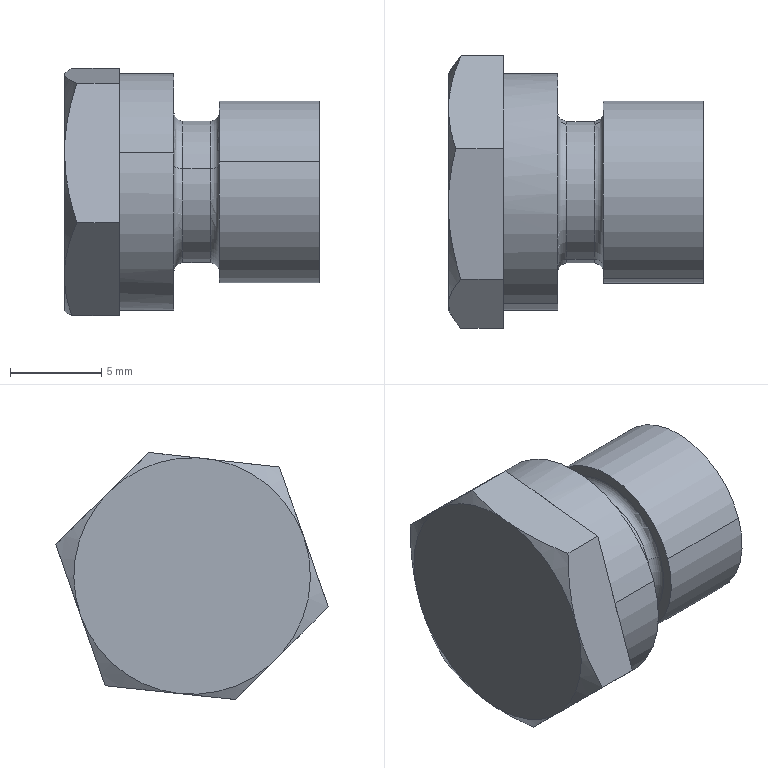Part | SolidWorks | features BaseBody 1 | 1 solid | 34 faces | box 14 x 14.972 x 13.575 mm | volume 1390 mm3 | plane 18 | cylinder 6 | cone 6 | torus 4 | commonest cylinder face diameters 7.8 x2 10 x2 13 x2
STEP:
#1=CARTESIAN_POINT('',(-79.963,84.032,-204.194));
#2=VERTEX_POINT('',#1);
#3=CARTESIAN_POINT('',(-79.963,71.76,-199.906));
#4=VERTEX_POINT('',#3);
#5=CARTESIAN_POINT('',(-79.963,77.896,-202.05));
#6=DIRECTION('',(1.,0.,0.));
#7=DIRECTION('',(0.,0.944,-0.3299));
#8=AXIS2_PLACEMENT_3D('',#5,#6,#7);
#9=CIRCLE('',#8,6.5);
#10=EDGE_CURVE('',#2,#4,#9,.T.);
#11=ORIENTED_EDGE('',*,*,#10,.F.);
#12=CARTESIAN_POINT('',(-82.963,84.032,-204.194));
#13=VERTEX_POINT('',#12);
#14=CARTESIAN_POINT('',(-79.963,84.032,-204.194));
#15=DIRECTION('',(-1.,0.,0.));
#16=VECTOR('',#15,1000.);
#17=LINE('',#14,#16);
#18=EDGE_CURVE('',#2,#13,#17,.T.);
#19=ORIENTED_EDGE('',*,*,#18,.T.);
#20=CARTESIAN_POINT('',(-82.963,82.458,-197.419));
#21=VERTEX_POINT('',#20);
#22=CARTESIAN_POINT('',(-82.963,77.896,-202.05));
#23=DIRECTION('',(1.,0.,0.));
#24=DIRECTION('',(0.,0.944,-0.3299));
#25=AXIS2_PLACEMENT_3D('',#22,#23,#24);
#26=CIRCLE('',#25,6.5);
#27=EDGE_CURVE('',#13,#21,#26,.T.);
#28=ORIENTED_EDGE('',*,*,#27,.T.);
#29=CARTESIAN_POINT('',(-82.963,77.67,-195.554));
#30=VERTEX_POINT('',#29);
#31=CARTESIAN_POINT('',(-82.963,77.896,-202.05));
#32=DIRECTION('',(1.,0.,0.));
#33=DIRECTION('',(0.,0.944,-0.3299));
#34=AXIS2_PLACEMENT_3D('',#31,#32,#33);
#35=CIRCLE('',#34,6.5);
#36=EDGE_CURVE('',#21,#30,#35,.T.);
#37=ORIENTED_EDGE('',*,*,#36,.T.);
#38=CARTESIAN_POINT('',(-82.963,76.677,-195.665));
#39=VERTEX_POINT('',#38);
#40=CARTESIAN_POINT('',(-82.963,77.896,-202.05));
#41=DIRECTION('',(1.,0.,0.));
#42=DIRECTION('',(0.,0.944,-0.3299));
#43=AXIS2_PLACEMENT_3D('',#40,#41,#42);
#44=CIRCLE('',#43,6.5);
#45=EDGE_CURVE('',#30,#39,#44,.T.);
#46=ORIENTED_EDGE('',*,*,#45,.T.);
#47=CARTESIAN_POINT('',(-82.963,71.76,-199.906));
#48=VERTEX_POINT('',#47);
#49=CARTESIAN_POINT('',(-82.963,77.896,-202.05));
#50=DIRECTION('',(1.,0.,0.));
#51=DIRECTION('',(0.,0.944,-0.3299));
#52=AXIS2_PLACEMENT_3D('',#49,#50,#51);
#53=CIRCLE('',#52,6.5);
#54=EDGE_CURVE('',#39,#48,#53,.T.);
#55=ORIENTED_EDGE('',*,*,#54,.T.);
#56=CARTESIAN_POINT('',(-79.963,71.76,-199.906));
#57=DIRECTION('',(-1.,0.,0.));
#58=VECTOR('',#57,1000.);
#59=LINE('',#56,#58);
#60=EDGE_CURVE('',#4,#48,#59,.T.);
#61=ORIENTED_EDGE('',*,*,#60,.F.);
#62=EDGE_LOOP('',(#11,#19,#28,#37,#46,#55,#61));
#63=FACE_OUTER_BOUND('',#62,.T.);
#64=CARTESIAN_POINT('',(-79.963,77.896,-202.05));
#65=DIRECTION('',(-1.,0.,0.));
#66=DIRECTION('',(0.,-0.944,0.3299));
#67=AXIS2_PLACEMENT_3D('',#64,#65,#66);
#68=CYLINDRICAL_SURFACE('',#67,6.5);
#69=ADVANCED_FACE('',(#63),#68,.T.);
#70=CARTESIAN_POINT('',(-77.963,74.215,-200.763));
#71=VERTEX_POINT('',#70);
#72=CARTESIAN_POINT('',(-77.963,81.578,-203.337));
#73=VERTEX_POINT('',#72);
#74=CARTESIAN_POINT('',(-77.963,77.896,-202.05));
#75=DIRECTION('',(-1.,0.,0.));
#76=DIRECTION('',(0.,0.944,-0.3299));
#77=AXIS2_PLACEMENT_3D('',#74,#75,#76);
#78=CIRCLE('',#77,3.9);
#79=EDGE_CURVE('',#71,#73,#78,.T.);
#80=ORIENTED_EDGE('',*,*,#79,.T.);
#81=CARTESIAN_POINT('',(-79.463,81.578,-203.337));
#82=VERTEX_POINT('',#81);
#83=CARTESIAN_POINT('',(-77.463,81.578,-203.337));
#84=DIRECTION('',(-1.,0.,0.));
#85=VECTOR('',#84,1000.);
#86=LINE('',#83,#85);
#87=EDGE_CURVE('',#73,#82,#86,.T.);
#88=ORIENTED_EDGE('',*,*,#87,.T.);
#89=CARTESIAN_POINT('',(-79.463,74.215,-200.763));
#90=VERTEX_POINT('',#89);
#91=CARTESIAN_POINT('',(-79.463,77.896,-202.05));
#92=DIRECTION('',(1.,0.,0.));
#93=DIRECTION('',(0.,0.944,-0.3299));
#94=AXIS2_PLACEMENT_3D('',#91,#92,#93);
#95=CIRCLE('',#94,3.9);
#96=EDGE_CURVE('',#82,#90,#95,.T.);
#97=ORIENTED_EDGE('',*,*,#96,.T.);
#98=CARTESIAN_POINT('',(-77.463,74.215,-200.763));
#99=DIRECTION('',(-1.,0.,0.));
#100=VECTOR('',#99,1000.);
#101=LINE('',#98,#100);
#102=EDGE_CURVE('',#71,#90,#101,.T.);
#103=ORIENTED_EDGE('',*,*,#102,.F.);
#104=EDGE_LOOP('',(#80,#88,#97,#103));
#105=FACE_OUTER_BOUND('',#104,.T.);
#106=CARTESIAN_POINT('',(-77.463,77.896,-202.05));
#107=DIRECTION('',(-1.,0.,0.));
#108=DIRECTION('',(0.,-0.944,0.3299));
#109=AXIS2_PLACEMENT_3D('',#106,#107,#108);
#110=CYLINDRICAL_SURFACE('',#109,3.9);
#111=ADVANCED_FACE('',(#105),#110,.T.);
#112=CARTESIAN_POINT('',(-71.963,82.616,-203.699));
#113=VERTEX_POINT('',#112);
#114=CARTESIAN_POINT('',(-71.963,73.176,-200.401));
#115=VERTEX_POINT('',#114);
#116=CARTESIAN_POINT('',(-71.963,77.896,-202.05));
#117=DIRECTION('',(1.,0.,0.));
#118=DIRECTION('',(0.,0.944,-0.3299));
#119=AXIS2_PLACEMENT_3D('',#116,#117,#118);
#120=CIRCLE('',#119,5.);
#121=EDGE_CURVE('',#113,#115,#120,.T.);
#122=ORIENTED_EDGE('',*,*,#121,.F.);
#123=CARTESIAN_POINT('',(-77.463,82.616,-203.699));
#124=VERTEX_POINT('',#123);
#125=CARTESIAN_POINT('',(-71.963,82.616,-203.699));
#126=DIRECTION('',(-1.,0.,0.));
#127=VECTOR('',#126,1000.);
#128=LINE('',#125,#127);
#129=EDGE_CURVE('',#113,#124,#128,.T.);
#130=ORIENTED_EDGE('',*,*,#129,.T.);
#131=CARTESIAN_POINT('',(-77.463,73.176,-200.401));
#132=VERTEX_POINT('',#131);
#133=CARTESIAN_POINT('',(-77.463,77.896,-202.05));
#134=DIRECTION('',(1.,0.,0.));
#135=DIRECTION('',(0.,0.944,-0.3299));
#136=AXIS2_PLACEMENT_3D('',#133,#134,#135);
#137=CIRCLE('',#136,5.);
#138=EDGE_CURVE('',#124,#132,#137,.T.);
#139=ORIENTED_EDGE('',*,*,#138,.T.);
#140=CARTESIAN_POINT('',(-71.963,73.176,-200.401));
#141=DIRECTION('',(-1.,0.,0.));
#142=VECTOR('',#141,1000.);
#143=LINE('',#140,#142);
#144=EDGE_CURVE('',#115,#132,#143,.T.);
#145=ORIENTED_EDGE('',*,*,#144,.F.);
#146=EDGE_LOOP('',(#122,#130,#139,#145));
#147=FACE_OUTER_BOUND('',#146,.T.);
#148=CARTESIAN_POINT('',(-71.963,77.896,-202.05));
#149=DIRECTION('',(-1.,0.,0.));
#150=DIRECTION('',(0.,-0.944,0.3299));
#151=AXIS2_PLACEMENT_3D('',#148,#149,#150);
#152=CYLINDRICAL_SURFACE('',#151,5.);
#153=ADVANCED_FACE('',(#147),#152,.T.);
#154=CARTESIAN_POINT('',(-79.463,77.896,-202.05));
#155=DIRECTION('',(1.,0.,0.));
#156=DIRECTION('',(0.,0.944,-0.3299));
#157=AXIS2_PLACEMENT_3D('',#154,#155,#156);
#158=CIRCLE('',#157,3.9);
#159=EDGE_CURVE('',#90,#82,#158,.T.);
#160=ORIENTED_EDGE('',*,*,#159,.F.);
#161=CARTESIAN_POINT('',(-79.963,73.743,-200.598));
#162=VERTEX_POINT('',#161);
#163=CARTESIAN_POINT('',(-79.463,73.743,-200.598));
#164=DIRECTION('',(0.,0.3299,0.944));
#165=DIRECTION('',(0.,-0.944,0.3299));
#166=AXIS2_PLACEMENT_3D('',#163,#164,#165);
#167=CIRCLE('',#166,0.5);
#168=EDGE_CURVE('',#90,#162,#167,.T.);
#169=ORIENTED_EDGE('',*,*,#168,.T.);
#170=CARTESIAN_POINT('',(-79.963,82.05,-203.502));
#171=VERTEX_POINT('',#170);
#172=CARTESIAN_POINT('',(-79.963,77.896,-202.05));
#173=DIRECTION('',(-1.,0.,0.));
#174=DIRECTION('',(0.,0.944,-0.3299));
#175=AXIS2_PLACEMENT_3D('',#172,#173,#174);
#176=CIRCLE('',#175,4.4);
#177=EDGE_CURVE('',#171,#162,#176,.T.);
#178=ORIENTED_EDGE('',*,*,#177,.F.);
#179=CARTESIAN_POINT('',(-79.463,82.05,-203.502));
#180=DIRECTION('',(0.,-0.3299,-0.944));
#181=DIRECTION('',(0.,0.944,-0.3299));
#182=AXIS2_PLACEMENT_3D('',#179,#180,#181);
#183=CIRCLE('',#182,0.5);
#184=EDGE_CURVE('',#82,#171,#183,.T.);
#185=ORIENTED_EDGE('',*,*,#184,.F.);
#186=EDGE_LOOP('',(#160,#169,#178,#185));
#187=FACE_OUTER_BOUND('',#186,.T.);
#188=CARTESIAN_POINT('',(-79.463,77.896,-202.05));
#189=DIRECTION('',(1.,0.,0.));
#190=DIRECTION('',(0.,0.944,-0.3299));
#191=AXIS2_PLACEMENT_3D('',#188,#189,#190);
#192=TOROIDAL_SURFACE('',#191,4.4,0.5);
#193=ADVANCED_FACE('',(#187),#192,.F.);
#194=CARTESIAN_POINT('',(-77.463,73.743,-200.598));
#195=VERTEX_POINT('',#194);
#196=CARTESIAN_POINT('',(-77.463,82.05,-203.502));
#197=VERTEX_POINT('',#196);
#198=CARTESIAN_POINT('',(-77.463,77.896,-202.05));
#199=DIRECTION('',(1.,0.,0.));
#200=DIRECTION('',(0.,0.944,-0.3299));
#201=AXIS2_PLACEMENT_3D('',#198,#199,#200);
#202=CIRCLE('',#201,4.4);
#203=EDGE_CURVE('',#195,#197,#202,.T.);
#204=ORIENTED_EDGE('',*,*,#203,.F.);
#205=CARTESIAN_POINT('',(-77.963,73.743,-200.598));
#206=DIRECTION('',(0.,0.3299,0.944));
#207=DIRECTION('',(0.,-0.944,0.3299));
#208=AXIS2_PLACEMENT_3D('',#205,#206,#207);
#209=CIRCLE('',#208,0.5);
#210=EDGE_CURVE('',#195,#71,#209,.T.);
#211=ORIENTED_EDGE('',*,*,#210,.T.);
#212=CARTESIAN_POINT('',(-77.963,77.896,-202.05));
#213=DIRECTION('',(-1.,0.,0.));
#214=DIRECTION('',(0.,0.944,-0.3299));
#215=AXIS2_PLACEMENT_3D('',#212,#213,#214);
#216=CIRCLE('',#215,3.9);
#217=EDGE_CURVE('',#73,#71,#216,.T.);
#218=ORIENTED_EDGE('',*,*,#217,.F.);
#219=CARTESIAN_POINT('',(-77.963,82.05,-203.502));
#220=DIRECTION('',(0.,-0.3299,-0.944));
#221=DIRECTION('',(0.,0.944,-0.3299));
#222=AXIS2_PLACEMENT_3D('',#219,#220,#221);
#223=CIRCLE('',#222,0.5);
#224=EDGE_CURVE('',#197,#73,#223,.T.);
#225=ORIENTED_EDGE('',*,*,#224,.F.);
#226=EDGE_LOOP('',(#204,#211,#218,#225));
#227=FACE_OUTER_BOUND('',#226,.T.);
#228=CARTESIAN_POINT('',(-77.963,77.896,-202.05));
#229=DIRECTION('',(1.,0.,0.));
#230=DIRECTION('',(0.,0.944,-0.3299));
#231=AXIS2_PLACEMENT_3D('',#228,#229,#230);
#232=TOROIDAL_SURFACE('',#231,4.4,0.5);
#233=ADVANCED_FACE('',(#227),#232,.F.);
#234=ORIENTED_EDGE('',*,*,#210,.F.);
#235=CARTESIAN_POINT('',(-77.463,77.896,-202.05));
#236=DIRECTION('',(1.,0.,0.));
#237=DIRECTION('',(0.,0.944,-0.3299));
#238=AXIS2_PLACEMENT_3D('',#235,#236,#237);
#239=CIRCLE('',#238,4.4);
#240=EDGE_CURVE('',#197,#195,#239,.T.);
#241=ORIENTED_EDGE('',*,*,#240,.F.);
#242=ORIENTED_EDGE('',*,*,#224,.T.);
#243=ORIENTED_EDGE('',*,*,#79,.F.);
#244=EDGE_LOOP('',(#234,#241,#242,#243));
#245=FACE_OUTER_BOUND('',#244,.T.);
#246=CARTESIAN_POINT('',(-77.963,77.896,-202.05));
#247=DIRECTION('',(1.,0.,0.));
#248=DIRECTION('',(0.,0.944,-0.3299));
#249=AXIS2_PLACEMENT_3D('',#246,#247,#248);
#250=TOROIDAL_SURFACE('',#249,4.4,0.5);
#251=ADVANCED_FACE('',(#245),#250,.F.);
#252=ORIENTED_EDGE('',*,*,#168,.F.);
#253=ORIENTED_EDGE('',*,*,#96,.F.);
#254=ORIENTED_EDGE('',*,*,#184,.T.);
#255=CARTESIAN_POINT('',(-79.963,77.896,-202.05));
#256=DIRECTION('',(-1.,0.,0.));
#257=DIRECTION('',(0.,0.944,-0.3299));
#258=AXIS2_PLACEMENT_3D('',#255,#256,#257);
#259=CIRCLE('',#258,4.4);
#260=EDGE_CURVE('',#162,#171,#259,.T.);
#261=ORIENTED_EDGE('',*,*,#260,.F.);
#262=EDGE_LOOP('',(#252,#253,#254,#261));
#263=FACE_OUTER_BOUND('',#262,.T.);
#264=CARTESIAN_POINT('',(-79.463,77.896,-202.05));
#265=DIRECTION('',(1.,0.,0.));
#266=DIRECTION('',(0.,0.944,-0.3299));
#267=AXIS2_PLACEMENT_3D('',#264,#265,#266);
#268=TOROIDAL_SURFACE('',#267,4.4,0.5);
#269=ADVANCED_FACE('',(#263),#268,.F.);
#270=CARTESIAN_POINT('',(-71.963,77.896,-202.05));
#271=DIRECTION('',(1.,0.,0.));
#272=DIRECTION('',(0.,0.944,-0.3299));
#273=AXIS2_PLACEMENT_3D('',#270,#271,#272);
#274=CIRCLE('',#273,5.);
#275=EDGE_CURVE('',#115,#113,#274,.T.);
#276=ORIENTED_EDGE('',*,*,#275,.T.);
#277=ORIENTED_EDGE('',*,*,#121,.T.);
#278=EDGE_LOOP('',(#276,#277));
#279=FACE_OUTER_BOUND('',#278,.T.);
#280=CARTESIAN_POINT('',(-71.963,77.896,-202.05));
#281=DIRECTION('',(1.,0.,0.));
#282=DIRECTION('',(0.,0.,-1.));
#283=AXIS2_PLACEMENT_3D('',#280,#281,#282);
#284=PLANE('',#283);
#285=ADVANCED_FACE('',(#279),#284,.T.);
#286=ORIENTED_EDGE('',*,*,#129,.F.);
#287=ORIENTED_EDGE('',*,*,#275,.F.);
#288=ORIENTED_EDGE('',*,*,#144,.T.);
#289=CARTESIAN_POINT('',(-77.463,77.896,-202.05));
#290=DIRECTION('',(1.,0.,0.));
#291=DIRECTION('',(0.,0.944,-0.3299));
#292=AXIS2_PLACEMENT_3D('',#289,#290,#291);
#293=CIRCLE('',#292,5.);
#294=EDGE_CURVE('',#132,#124,#293,.T.);
#295=ORIENTED_EDGE('',*,*,#294,.T.);
#296=EDGE_LOOP('',(#286,#287,#288,#295));
#297=FACE_OUTER_BOUND('',#296,.T.);
#298=CARTESIAN_POINT('',(-71.963,77.896,-202.05));
#299=DIRECTION('',(-1.,0.,0.));
#300=DIRECTION('',(0.,-0.944,0.3299));
#301=AXIS2_PLACEMENT_3D('',#298,#299,#300);
#302=CYLINDRICAL_SURFACE('',#301,5.);
#303=ADVANCED_FACE('',(#297),#302,.T.);
#304=ORIENTED_EDGE('',*,*,#294,.F.);
#305=ORIENTED_EDGE('',*,*,#138,.F.);
#306=EDGE_LOOP('',(#304,#305));
#307=FACE_OUTER_BOUND('',#306,.T.);
#308=ORIENTED_EDGE('',*,*,#240,.T.);
#309=ORIENTED_EDGE('',*,*,#203,.T.);
#310=EDGE_LOOP('',(#308,#309));
#311=FACE_BOUND('',#310,.T.);
#312=CARTESIAN_POINT('',(-77.463,77.896,-202.05));
#313=DIRECTION('',(1.,0.,0.));
#314=DIRECTION('',(0.,0.,-1.));
#315=AXIS2_PLACEMENT_3D('',#312,#313,#314);
#316=PLANE('',#315);
#317=ADVANCED_FACE('',(#307,#311),#316,.F.);
#318=ORIENTED_EDGE('',*,*,#87,.F.);
#319=ORIENTED_EDGE('',*,*,#217,.T.);
#320=ORIENTED_EDGE('',*,*,#102,.T.);
#321=ORIENTED_EDGE('',*,*,#159,.T.);
#322=EDGE_LOOP('',(#318,#319,#320,#321));
#323=FACE_OUTER_BOUND('',#322,.T.);
#324=CARTESIAN_POINT('',(-77.463,77.896,-202.05));
#325=DIRECTION('',(-1.,0.,0.));
#326=DIRECTION('',(0.,-0.944,0.3299));
#327=AXIS2_PLACEMENT_3D('',#324,#325,#326);
#328=CYLINDRICAL_SURFACE('',#327,3.9);
#329=ADVANCED_FACE('',(#323),#328,.T.);
#330=ORIENTED_EDGE('',*,*,#18,.F.);
#331=CARTESIAN_POINT('',(-79.963,77.896,-202.05));
#332=DIRECTION('',(1.,0.,0.));
#333=DIRECTION('',(0.,0.944,-0.3299));
#334=AXIS2_PLACEMENT_3D('',#331,#332,#333);
#335=CIRCLE('',#334,6.5);
#336=EDGE_CURVE('',#4,#2,#335,.T.);
#337=ORIENTED_EDGE('',*,*,#336,.F.);
#338=ORIENTED_EDGE('',*,*,#60,.T.);
#339=CARTESIAN_POINT('',(-82.963,72.966,-206.286));
#340=VERTEX_POINT('',#339);
#341=CARTESIAN_POINT('',(-82.963,77.896,-202.05));
#342=DIRECTION('',(1.,0.,0.));
#343=DIRECTION('',(0.,0.944,-0.3299));
#344=AXIS2_PLACEMENT_3D('',#341,#342,#343);
#345=CIRCLE('',#344,6.5);
#346=EDGE_CURVE('',#48,#340,#345,.T.);
#347=ORIENTED_EDGE('',*,*,#346,.T.);
#348=CARTESIAN_POINT('',(-82.963,73.673,-206.991));
#349=VERTEX_POINT('',#348);
#350=CARTESIAN_POINT('',(-82.963,77.896,-202.05));
#351=DIRECTION('',(1.,0.,0.));
#352=DIRECTION('',(0.,0.944,-0.3299));
#353=AXIS2_PLACEMENT_3D('',#350,#351,#352);
#354=CIRCLE('',#353,6.5);
#355=EDGE_CURVE('',#340,#349,#354,.T.);
#356=ORIENTED_EDGE('',*,*,#355,.T.);
#357=CARTESIAN_POINT('',(-82.963,78.581,-208.514));
#358=VERTEX_POINT('',#357);
#359=CARTESIAN_POINT('',(-82.963,77.896,-202.05));
#360=DIRECTION('',(1.,0.,0.));
#361=DIRECTION('',(0.,0.944,-0.3299));
#362=AXIS2_PLACEMENT_3D('',#359,#360,#361);
#363=CIRCLE('',#362,6.5);
#364=EDGE_CURVE('',#349,#358,#363,.T.);
#365=ORIENTED_EDGE('',*,*,#364,.T.);
#366=CARTESIAN_POINT('',(-82.963,77.896,-202.05));
#367=DIRECTION('',(1.,0.,0.));
#368=DIRECTION('',(0.,0.944,-0.3299));
#369=AXIS2_PLACEMENT_3D('',#366,#367,#368);
#370=CIRCLE('',#369,6.5);
#371=EDGE_CURVE('',#358,#13,#370,.T.);
#372=ORIENTED_EDGE('',*,*,#371,.T.);
#373=EDGE_LOOP('',(#330,#337,#338,#347,#356,#365,#372));
#374=FACE_OUTER_BOUND('',#373,.T.);
#375=CARTESIAN_POINT('',(-79.963,77.896,-202.05));
#376=DIRECTION('',(-1.,0.,0.));
#377=DIRECTION('',(0.,-0.944,0.3299));
#378=AXIS2_PLACEMENT_3D('',#375,#376,#377);
#379=CYLINDRICAL_SURFACE('',#378,6.5);
#380=ADVANCED_FACE('',(#374),#379,.T.);
#381=ORIENTED_EDGE('',*,*,#355,.F.);
#382=CARTESIAN_POINT('',(-82.963,75.524,-208.837));
#383=DIRECTION('',(0.,0.708,-0.7062));
#384=VECTOR('',#383,1000.);
#385=LINE('',#382,#384);
#386=EDGE_CURVE('',#340,#349,#385,.T.);
#387=ORIENTED_EDGE('',*,*,#386,.T.);
#388=EDGE_LOOP('',(#381,#387));
#389=FACE_OUTER_BOUND('',#388,.T.);
#390=CARTESIAN_POINT('',(-82.963,77.896,-202.05));
#391=DIRECTION('',(1.,0.,0.));
#392=DIRECTION('',(0.,0.,-1.));
#393=AXIS2_PLACEMENT_3D('',#390,#391,#392);
#394=PLANE('',#393);
#395=ADVANCED_FACE('',(#389),#394,.F.);
#396=ORIENTED_EDGE('',*,*,#45,.F.);
#397=CARTESIAN_POINT('',(-82.963,80.268,-195.263));
#398=DIRECTION('',(0.,-0.9938,-0.1115));
#399=VECTOR('',#398,1000.);
#400=LINE('',#397,#399);
#401=EDGE_CURVE('',#30,#39,#400,.T.);
#402=ORIENTED_EDGE('',*,*,#401,.T.);
#403=EDGE_LOOP('',(#396,#402));
#404=FACE_OUTER_BOUND('',#403,.T.);
#405=CARTESIAN_POINT('',(-82.963,77.896,-202.05));
#406=DIRECTION('',(1.,0.,0.));
#407=DIRECTION('',(0.,0.,-1.));
#408=AXIS2_PLACEMENT_3D('',#405,#406,#407);
#409=PLANE('',#408);
#410=ADVANCED_FACE('',(#404),#409,.F.);
#411=CARTESIAN_POINT('',(-85.289,70.418,-203.745));
#412=VERTEX_POINT('',#411);
#413=CARTESIAN_POINT('',(-85.963,71.76,-199.906));
#414=VERTEX_POINT('',#413);
#415=CARTESIAN_POINT('',(-85.289,70.418,-203.745));
#416=CARTESIAN_POINT('',(-85.492,70.637,-203.119));
#417=CARTESIAN_POINT('',(-85.661,70.858,-202.488));
#418=CARTESIAN_POINT('',(-85.897,71.304,-201.21));
#419=CARTESIAN_POINT('',(-85.963,71.53,-200.563));
#420=CARTESIAN_POINT('',(-85.963,71.76,-199.906));
#421=B_SPLINE_CURVE_WITH_KNOTS('',3,(#415,#416,#417,#418,#419,#420),.UNSPECIFIED.,.F.,.F.,(4,2,4),(0.,0.002061,0.004122),.UNSPECIFIED.);
#422=EDGE_CURVE('',#412,#414,#421,.T.);
#423=ORIENTED_EDGE('',*,*,#422,.T.);
#424=CARTESIAN_POINT('',(-85.963,72.966,-206.286));
#425=VERTEX_POINT('',#424);
#426=CARTESIAN_POINT('',(-85.963,77.896,-202.05));
#427=DIRECTION('',(1.,0.,0.));
#428=DIRECTION('',(0.,-0.944,0.3299));
#429=AXIS2_PLACEMENT_3D('',#426,#427,#428);
#430=CIRCLE('',#429,6.5);
#431=EDGE_CURVE('',#414,#425,#430,.T.);
#432=ORIENTED_EDGE('',*,*,#431,.T.);
#433=CARTESIAN_POINT('',(-85.963,72.966,-206.286));
#434=CARTESIAN_POINT('',(-85.908,72.094,-205.416));
#435=CARTESIAN_POINT('',(-85.651,71.249,-204.574));
#436=CARTESIAN_POINT('',(-85.289,70.418,-203.745));
#437=B_SPLINE_CURVE_WITH_KNOTS('',3,(#433,#434,#435,#436),.UNSPECIFIED.,.F.,.F.,(4,4),(0.,0.00366),.UNSPECIFIED.);
#438=EDGE_CURVE('',#425,#412,#437,.T.);
#439=ORIENTED_EDGE('',*,*,#438,.T.);
#440=EDGE_LOOP('',(#423,#432,#439));
#441=FACE_OUTER_BOUND('',#440,.T.);
#442=CARTESIAN_POINT('',(-85.963,77.896,-202.05));
#443=DIRECTION('',(1.,0.,0.));
#444=DIRECTION('',(0.,-0.944,0.3299));
#445=AXIS2_PLACEMENT_3D('',#442,#443,#444);
#446=CONICAL_SURFACE('',#445,6.5,1.047);
#447=ADVANCED_FACE('',(#441),#446,.T.);
#448=CARTESIAN_POINT('',(-85.565,75.524,-208.837));
#449=VERTEX_POINT('',#448);
#450=CARTESIAN_POINT('',(-85.963,73.673,-206.991));
#451=VERTEX_POINT('',#450);
#452=CARTESIAN_POINT('',(-85.565,75.524,-208.837));
#453=CARTESIAN_POINT('',(-85.779,74.916,-208.231));
#454=CARTESIAN_POINT('',(-85.924,74.3,-207.617));
#455=CARTESIAN_POINT('',(-85.963,73.673,-206.991));
#456=B_SPLINE_CURVE_WITH_KNOTS('',3,(#452,#453,#454,#455),.UNSPECIFIED.,.F.,.F.,(4,4),(0.,0.002644),.UNSPECIFIED.);
#457=EDGE_CURVE('',#449,#451,#456,.T.);
#458=ORIENTED_EDGE('',*,*,#457,.T.);
#459=CARTESIAN_POINT('',(-85.963,78.581,-208.514));
#460=VERTEX_POINT('',#459);
#461=CARTESIAN_POINT('',(-85.963,77.896,-202.05));
#462=DIRECTION('',(1.,0.,0.));
#463=DIRECTION('',(0.,-0.944,0.3299));
#464=AXIS2_PLACEMENT_3D('',#461,#462,#463);
#465=CIRCLE('',#464,6.5);
#466=EDGE_CURVE('',#451,#460,#465,.T.);
#467=ORIENTED_EDGE('',*,*,#466,.T.);
#468=CARTESIAN_POINT('',(-85.963,78.581,-208.514));
#469=CARTESIAN_POINT('',(-85.963,77.545,-208.624));
#470=CARTESIAN_POINT('',(-85.814,76.528,-208.731));
#471=CARTESIAN_POINT('',(-85.565,75.524,-208.837));
#472=B_SPLINE_CURVE_WITH_KNOTS('',3,(#468,#469,#470,#471),.UNSPECIFIED.,.F.,.F.,(4,4),(0.,0.003099),.UNSPECIFIED.);
#473=EDGE_CURVE('',#460,#449,#472,.T.);
#474=ORIENTED_EDGE('',*,*,#473,.T.);
#475=EDGE_LOOP('',(#458,#467,#474));
#476=FACE_OUTER_BOUND('',#475,.T.);
#477=CARTESIAN_POINT('',(-85.963,77.896,-202.05));
#478=DIRECTION('',(1.,0.,0.));
#479=DIRECTION('',(0.,-0.944,0.3299));
#480=AXIS2_PLACEMENT_3D('',#477,#478,#479);
#481=CONICAL_SURFACE('',#480,6.5,1.047);
#482=ADVANCED_FACE('',(#476),#481,.T.);
#483=CARTESIAN_POINT('',(-85.274,82.674,-208.08));
#484=VERTEX_POINT('',#483);
#485=CARTESIAN_POINT('',(-85.274,82.674,-208.08));
#486=CARTESIAN_POINT('',(-85.481,82.007,-208.151));
#487=CARTESIAN_POINT('',(-85.654,81.335,-208.222));
#488=CARTESIAN_POINT('',(-85.895,79.972,-208.367));
#489=CARTESIAN_POINT('',(-85.963,79.282,-208.44));
#490=CARTESIAN_POINT('',(-85.963,78.581,-208.514));
#491=B_SPLINE_CURVE_WITH_KNOTS('',3,(#485,#486,#487,#488,#489,#490),.UNSPECIFIED.,.F.,.F.,(4,2,4),(0.,0.002087,0.004174),.UNSPECIFIED.);
#492=EDGE_CURVE('',#484,#460,#491,.T.);
#493=ORIENTED_EDGE('',*,*,#492,.T.);
#494=CARTESIAN_POINT('',(-85.963,84.032,-204.194));
#495=VERTEX_POINT('',#494);
#496=CARTESIAN_POINT('',(-85.963,77.896,-202.05));
#497=DIRECTION('',(1.,0.,0.));
#498=DIRECTION('',(0.,-0.944,0.3299));
#499=AXIS2_PLACEMENT_3D('',#496,#497,#498);
#500=CIRCLE('',#499,6.5);
#501=EDGE_CURVE('',#460,#495,#500,.T.);
#502=ORIENTED_EDGE('',*,*,#501,.T.);
#503=CARTESIAN_POINT('',(-85.963,84.032,-204.194));
#504=CARTESIAN_POINT('',(-85.963,83.8,-204.86));
#505=CARTESIAN_POINT('',(-85.895,83.571,-205.515));
#506=CARTESIAN_POINT('',(-85.654,83.119,-206.809));
#507=CARTESIAN_POINT('',(-85.481,82.896,-207.447));
#508=CARTESIAN_POINT('',(-85.274,82.674,-208.08));
#509=B_SPLINE_CURVE_WITH_KNOTS('',3,(#503,#504,#505,#506,#507,#508),.UNSPECIFIED.,.F.,.F.,(4,2,4),(0.,0.002087,0.004174),.UNSPECIFIED.);
#510=EDGE_CURVE('',#495,#484,#509,.T.);
#511=ORIENTED_EDGE('',*,*,#510,.T.);
#512=EDGE_LOOP('',(#493,#502,#511));
#513=FACE_OUTER_BOUND('',#512,.T.);
#514=CARTESIAN_POINT('',(-85.963,77.896,-202.05));
#515=DIRECTION('',(1.,0.,0.));
#516=DIRECTION('',(0.,-0.944,0.3299));
#517=AXIS2_PLACEMENT_3D('',#514,#515,#516);
#518=CONICAL_SURFACE('',#517,6.5,1.047);
#519=ADVANCED_FACE('',(#513),#518,.T.);
#520=CARTESIAN_POINT('',(-85.274,85.39,-200.308));
#521=VERTEX_POINT('',#520);
#522=CARTESIAN_POINT('',(-85.274,85.39,-200.308));
#523=CARTESIAN_POINT('',(-85.481,85.169,-200.941));
#524=CARTESIAN_POINT('',(-85.654,84.946,-201.58));
#525=CARTESIAN_POINT('',(-85.895,84.494,-202.873));
#526=CARTESIAN_POINT('',(-85.963,84.265,-203.528));
#527=CARTESIAN_POINT('',(-85.963,84.032,-204.194));
#528=B_SPLINE_CURVE_WITH_KNOTS('',3,(#522,#523,#524,#525,#526,#527),.UNSPECIFIED.,.F.,.F.,(4,2,4),(0.,0.002087,0.004174),.UNSPECIFIED.);
#529=EDGE_CURVE('',#521,#495,#528,.T.);
#530=ORIENTED_EDGE('',*,*,#529,.T.);
#531=CARTESIAN_POINT('',(-85.963,82.458,-197.419));
#532=VERTEX_POINT('',#531);
#533=CARTESIAN_POINT('',(-85.963,77.896,-202.05));
#534=DIRECTION('',(1.,0.,0.));
#535=DIRECTION('',(0.,-0.944,0.3299));
#536=AXIS2_PLACEMENT_3D('',#533,#534,#535);
#537=CIRCLE('',#536,6.5);
#538=EDGE_CURVE('',#495,#532,#537,.T.);
#539=ORIENTED_EDGE('',*,*,#538,.T.);
#540=CARTESIAN_POINT('',(-85.963,82.458,-197.419));
#541=CARTESIAN_POINT('',(-85.963,82.96,-197.914));
#542=CARTESIAN_POINT('',(-85.895,83.455,-198.401));
#543=CARTESIAN_POINT('',(-85.654,84.431,-199.363));
#544=CARTESIAN_POINT('',(-85.481,84.913,-199.838));
#545=CARTESIAN_POINT('',(-85.274,85.39,-200.308));
#546=B_SPLINE_CURVE_WITH_KNOTS('',3,(#540,#541,#542,#543,#544,#545),.UNSPECIFIED.,.F.,.F.,(4,2,4),(0.,0.002087,0.004174),.UNSPECIFIED.);
#547=EDGE_CURVE('',#532,#521,#546,.T.);
#548=ORIENTED_EDGE('',*,*,#547,.T.);
#549=EDGE_LOOP('',(#530,#539,#548));
#550=FACE_OUTER_BOUND('',#549,.T.);
#551=CARTESIAN_POINT('',(-85.963,77.896,-202.05));
#552=DIRECTION('',(1.,0.,0.));
#553=DIRECTION('',(0.,-0.944,0.3299));
#554=AXIS2_PLACEMENT_3D('',#551,#552,#553);
#555=CONICAL_SURFACE('',#554,6.5,1.047);
#556=ADVANCED_FACE('',(#550),#555,.T.);
#557=CARTESIAN_POINT('',(-85.963,77.67,-195.554));
#558=VERTEX_POINT('',#557);
#559=CARTESIAN_POINT('',(-85.565,80.268,-195.263));
#560=VERTEX_POINT('',#559);
#561=CARTESIAN_POINT('',(-85.963,77.67,-195.554));
#562=CARTESIAN_POINT('',(-85.924,78.551,-195.455));
#563=CARTESIAN_POINT('',(-85.779,79.415,-195.358));
#564=CARTESIAN_POINT('',(-85.565,80.268,-195.263));
#565=B_SPLINE_CURVE_WITH_KNOTS('',3,(#561,#562,#563,#564),.UNSPECIFIED.,.F.,.F.,(4,4),(0.,0.002644),.UNSPECIFIED.);
#566=EDGE_CURVE('',#558,#560,#565,.T.);
#567=ORIENTED_EDGE('',*,*,#566,.T.);
#568=CARTESIAN_POINT('',(-85.565,80.268,-195.263));
#569=CARTESIAN_POINT('',(-85.814,80.987,-195.971));
#570=CARTESIAN_POINT('',(-85.963,81.716,-196.688));
#571=CARTESIAN_POINT('',(-85.963,82.458,-197.419));
#572=B_SPLINE_CURVE_WITH_KNOTS('',3,(#568,#569,#570,#571),.UNSPECIFIED.,.F.,.F.,(4,4),(0.,0.003099),.UNSPECIFIED.);
#573=EDGE_CURVE('',#560,#532,#572,.T.);
#574=ORIENTED_EDGE('',*,*,#573,.T.);
#575=CARTESIAN_POINT('',(-85.963,77.896,-202.05));
#576=DIRECTION('',(1.,0.,0.));
#577=DIRECTION('',(0.,-0.944,0.3299));
#578=AXIS2_PLACEMENT_3D('',#575,#576,#577);
#579=CIRCLE('',#578,6.5);
#580=EDGE_CURVE('',#532,#558,#579,.T.);
#581=ORIENTED_EDGE('',*,*,#580,.T.);
#582=EDGE_LOOP('',(#567,#574,#581));
#583=FACE_OUTER_BOUND('',#582,.T.);
#584=CARTESIAN_POINT('',(-85.963,77.896,-202.05));
#585=DIRECTION('',(1.,0.,0.));
#586=DIRECTION('',(0.,-0.944,0.3299));
#587=AXIS2_PLACEMENT_3D('',#584,#585,#586);
#588=CONICAL_SURFACE('',#587,6.5,1.047);
#589=ADVANCED_FACE('',(#583),#588,.T.);
#590=CARTESIAN_POINT('',(-85.289,73.102,-196.066));
#591=VERTEX_POINT('',#590);
#592=CARTESIAN_POINT('',(-85.963,76.677,-195.665));
#593=VERTEX_POINT('',#592);
#594=CARTESIAN_POINT('',(-85.289,73.102,-196.066));
#595=CARTESIAN_POINT('',(-85.651,74.268,-195.936));
#596=CARTESIAN_POINT('',(-85.908,75.454,-195.803));
#597=CARTESIAN_POINT('',(-85.963,76.677,-195.665));
#598=B_SPLINE_CURVE_WITH_KNOTS('',3,(#594,#595,#596,#597),.UNSPECIFIED.,.F.,.F.,(4,4),(0.,0.00366),.UNSPECIFIED.);
#599=EDGE_CURVE('',#591,#593,#598,.T.);
#600=ORIENTED_EDGE('',*,*,#599,.T.);
#601=CARTESIAN_POINT('',(-85.963,77.896,-202.05));
#602=DIRECTION('',(-1.,0.,0.));
#603=DIRECTION('',(0.,-0.944,0.3299));
#604=AXIS2_PLACEMENT_3D('',#601,#602,#603);
#605=CIRCLE('',#604,6.5);
#606=EDGE_CURVE('',#414,#593,#605,.T.);
#607=ORIENTED_EDGE('',*,*,#606,.F.);
#608=CARTESIAN_POINT('',(-85.963,71.76,-199.906));
#609=CARTESIAN_POINT('',(-85.963,71.99,-199.248));
#610=CARTESIAN_POINT('',(-85.897,72.216,-198.601));
#611=CARTESIAN_POINT('',(-85.661,72.663,-197.323));
#612=CARTESIAN_POINT('',(-85.492,72.883,-196.692));
#613=CARTESIAN_POINT('',(-85.289,73.102,-196.066));
#614=B_SPLINE_CURVE_WITH_KNOTS('',3,(#608,#609,#610,#611,#612,#613),.UNSPECIFIED.,.F.,.F.,(4,2,4),(0.,0.002061,0.004122),.UNSPECIFIED.);
#615=EDGE_CURVE('',#414,#591,#614,.T.);
#616=ORIENTED_EDGE('',*,*,#615,.T.);
#617=EDGE_LOOP('',(#600,#607,#616));
#618=FACE_OUTER_BOUND('',#617,.T.);
#619=CARTESIAN_POINT('',(-85.963,77.896,-202.05));
#620=DIRECTION('',(1.,0.,0.));
#621=DIRECTION('',(0.,-0.944,0.3299));
#622=AXIS2_PLACEMENT_3D('',#619,#620,#621);
#623=CONICAL_SURFACE('',#622,6.5,1.047);
#624=ADVANCED_FACE('',(#618),#623,.T.);
#625=ORIENTED_EDGE('',*,*,#466,.F.);
#626=CARTESIAN_POINT('',(-85.963,75.524,-208.837));
#627=DIRECTION('',(0.,0.708,-0.7062));
#628=VECTOR('',#627,1000.);
#629=LINE('',#626,#628);
#630=EDGE_CURVE('',#425,#451,#629,.T.);
#631=ORIENTED_EDGE('',*,*,#630,.F.);
#632=ORIENTED_EDGE('',*,*,#431,.F.);
#633=ORIENTED_EDGE('',*,*,#606,.T.);
#634=CARTESIAN_POINT('',(-85.963,80.268,-195.263));
#635=DIRECTION('',(0.,-0.9938,-0.1115));
#636=VECTOR('',#635,1000.);
#637=LINE('',#634,#636);
#638=EDGE_CURVE('',#558,#593,#637,.T.);
#639=ORIENTED_EDGE('',*,*,#638,.F.);
#640=ORIENTED_EDGE('',*,*,#580,.F.);
#641=ORIENTED_EDGE('',*,*,#538,.F.);
#642=ORIENTED_EDGE('',*,*,#501,.F.);
#643=EDGE_LOOP('',(#625,#631,#632,#633,#639,#640,#641,#642));
#644=FACE_OUTER_BOUND('',#643,.T.);
#645=CARTESIAN_POINT('',(-85.963,73.102,-196.066));
#646=DIRECTION('',(-1.,0.,0.));
#647=DIRECTION('',(0.,1.,0.));
#648=AXIS2_PLACEMENT_3D('',#645,#646,#647);
#649=PLANE('',#648);
#650=ADVANCED_FACE('',(#644),#649,.T.);
#651=ORIENTED_EDGE('',*,*,#573,.F.);
#652=CARTESIAN_POINT('',(-82.963,80.268,-195.263));
#653=VERTEX_POINT('',#652);
#654=CARTESIAN_POINT('',(-82.963,80.268,-195.263));
#655=DIRECTION('',(-1.,0.,0.));
#656=VECTOR('',#655,1000.);
#657=LINE('',#654,#656);
#658=EDGE_CURVE('',#653,#560,#657,.T.);
#659=ORIENTED_EDGE('',*,*,#658,.F.);
#660=CARTESIAN_POINT('',(-82.963,80.268,-195.263));
#661=DIRECTION('',(0.,-0.7124,0.7018));
#662=VECTOR('',#661,1000.);
#663=LINE('',#660,#662);
#664=EDGE_CURVE('',#21,#653,#663,.T.);
#665=ORIENTED_EDGE('',*,*,#664,.F.);
#666=CARTESIAN_POINT('',(-82.963,85.39,-200.308));
#667=VERTEX_POINT('',#666);
#668=CARTESIAN_POINT('',(-82.963,80.268,-195.263));
#669=DIRECTION('',(0.,-0.7124,0.7018));
#670=VECTOR('',#669,1000.);
#671=LINE('',#668,#670);
#672=EDGE_CURVE('',#667,#21,#671,.T.);
#673=ORIENTED_EDGE('',*,*,#672,.F.);
#674=CARTESIAN_POINT('',(-82.963,85.39,-200.308));
#675=DIRECTION('',(-1.,0.,0.));
#676=VECTOR('',#675,1000.);
#677=LINE('',#674,#676);
#678=EDGE_CURVE('',#667,#521,#677,.T.);
#679=ORIENTED_EDGE('',*,*,#678,.T.);
#680=ORIENTED_EDGE('',*,*,#547,.F.);
#681=EDGE_LOOP('',(#651,#659,#665,#673,#679,#680));
#682=FACE_OUTER_BOUND('',#681,.T.);
#683=CARTESIAN_POINT('',(-82.963,80.268,-195.263));
#684=DIRECTION('',(0.,-0.7018,-0.7124));
#685=DIRECTION('',(0.,-0.7124,0.7018));
#686=AXIS2_PLACEMENT_3D('',#683,#684,#685);
#687=PLANE('',#686);
#688=ADVANCED_FACE('',(#682),#687,.F.);
#689=ORIENTED_EDGE('',*,*,#529,.F.);
#690=ORIENTED_EDGE('',*,*,#678,.F.);
#691=CARTESIAN_POINT('',(-82.963,82.674,-208.08));
#692=DIRECTION('',(0.,0.3299,0.944));
#693=VECTOR('',#692,1000.);
#694=LINE('',#691,#693);
#695=EDGE_CURVE('',#13,#667,#694,.T.);
#696=ORIENTED_EDGE('',*,*,#695,.F.);
#697=CARTESIAN_POINT('',(-82.963,82.674,-208.08));
#698=VERTEX_POINT('',#697);
#699=CARTESIAN_POINT('',(-82.963,82.674,-208.08));
#700=DIRECTION('',(0.,0.3299,0.944));
#701=VECTOR('',#700,1000.);
#702=LINE('',#699,#701);
#703=EDGE_CURVE('',#698,#13,#702,.T.);
#704=ORIENTED_EDGE('',*,*,#703,.F.);
#705=CARTESIAN_POINT('',(-82.963,82.674,-208.08));
#706=DIRECTION('',(-1.,0.,0.));
#707=VECTOR('',#706,1000.);
#708=LINE('',#705,#707);
#709=EDGE_CURVE('',#698,#484,#708,.T.);
#710=ORIENTED_EDGE('',*,*,#709,.T.);
#711=ORIENTED_EDGE('',*,*,#510,.F.);
#712=EDGE_LOOP('',(#689,#690,#696,#704,#710,#711));
#713=FACE_OUTER_BOUND('',#712,.T.);
#714=CARTESIAN_POINT('',(-82.963,82.674,-208.08));
#715=DIRECTION('',(0.,-0.944,0.3299));
#716=DIRECTION('',(-1.,0.,0.));
#717=AXIS2_PLACEMENT_3D('',#714,#715,#716);
#718=PLANE('',#717);
#719=ADVANCED_FACE('',(#713),#718,.F.);
#720=ORIENTED_EDGE('',*,*,#492,.F.);
#721=ORIENTED_EDGE('',*,*,#709,.F.);
#722=CARTESIAN_POINT('',(-82.963,75.524,-208.837));
#723=DIRECTION('',(0.,0.9944,0.1053));
#724=VECTOR('',#723,1000.);
#725=LINE('',#722,#724);
#726=EDGE_CURVE('',#358,#698,#725,.T.);
#727=ORIENTED_EDGE('',*,*,#726,.F.);
#728=CARTESIAN_POINT('',(-82.963,75.524,-208.837));
#729=VERTEX_POINT('',#728);
#730=CARTESIAN_POINT('',(-82.963,75.524,-208.837));
#731=DIRECTION('',(0.,0.9944,0.1053));
#732=VECTOR('',#731,1000.);
#733=LINE('',#730,#732);
#734=EDGE_CURVE('',#729,#358,#733,.T.);
#735=ORIENTED_EDGE('',*,*,#734,.F.);
#736=CARTESIAN_POINT('',(-82.963,75.524,-208.837));
#737=DIRECTION('',(-1.,0.,0.));
#738=VECTOR('',#737,1000.);
#739=LINE('',#736,#738);
#740=EDGE_CURVE('',#729,#449,#739,.T.);
#741=ORIENTED_EDGE('',*,*,#740,.T.);
#742=ORIENTED_EDGE('',*,*,#473,.F.);
#743=EDGE_LOOP('',(#720,#721,#727,#735,#741,#742));
#744=FACE_OUTER_BOUND('',#743,.T.);
#745=CARTESIAN_POINT('',(-82.963,75.524,-208.837));
#746=DIRECTION('',(0.,-0.1053,0.9944));
#747=DIRECTION('',(-1.,0.,0.));
#748=AXIS2_PLACEMENT_3D('',#745,#746,#747);
#749=PLANE('',#748);
#750=ADVANCED_FACE('',(#744),#749,.F.);
#751=ORIENTED_EDGE('',*,*,#438,.F.);
#752=ORIENTED_EDGE('',*,*,#630,.T.);
#753=ORIENTED_EDGE('',*,*,#457,.F.);
#754=ORIENTED_EDGE('',*,*,#740,.F.);
#755=CARTESIAN_POINT('',(-82.963,75.524,-208.837));
#756=DIRECTION('',(0.,0.708,-0.7062));
#757=VECTOR('',#756,1000.);
#758=LINE('',#755,#757);
#759=EDGE_CURVE('',#349,#729,#758,.T.);
#760=ORIENTED_EDGE('',*,*,#759,.F.);
#761=ORIENTED_EDGE('',*,*,#386,.F.);
#762=CARTESIAN_POINT('',(-82.963,70.418,-203.745));
#763=VERTEX_POINT('',#762);
#764=CARTESIAN_POINT('',(-82.963,75.524,-208.837));
#765=DIRECTION('',(0.,0.708,-0.7062));
#766=VECTOR('',#765,1000.);
#767=LINE('',#764,#766);
#768=EDGE_CURVE('',#763,#340,#767,.T.);
#769=ORIENTED_EDGE('',*,*,#768,.F.);
#770=CARTESIAN_POINT('',(-82.963,70.418,-203.745));
#771=DIRECTION('',(-1.,0.,0.));
#772=VECTOR('',#771,1000.);
#773=LINE('',#770,#772);
#774=EDGE_CURVE('',#763,#412,#773,.T.);
#775=ORIENTED_EDGE('',*,*,#774,.T.);
#776=EDGE_LOOP('',(#751,#752,#753,#754,#760,#761,#769,#775));
#777=FACE_OUTER_BOUND('',#776,.T.);
#778=CARTESIAN_POINT('',(-82.963,75.524,-208.837));
#779=DIRECTION('',(0.,0.7062,0.708));
#780=DIRECTION('',(1.,0.,0.));
#781=AXIS2_PLACEMENT_3D('',#778,#779,#780);
#782=PLANE('',#781);
#783=ADVANCED_FACE('',(#777),#782,.F.);
#784=ORIENTED_EDGE('',*,*,#422,.F.);
#785=ORIENTED_EDGE('',*,*,#774,.F.);
#786=CARTESIAN_POINT('',(-82.963,70.418,-203.745));
#787=DIRECTION('',(0.,-0.3299,-0.944));
#788=VECTOR('',#787,1000.);
#789=LINE('',#786,#788);
#790=EDGE_CURVE('',#48,#763,#789,.T.);
#791=ORIENTED_EDGE('',*,*,#790,.F.);
#792=CARTESIAN_POINT('',(-82.963,73.102,-196.066));
#793=VERTEX_POINT('',#792);
#794=CARTESIAN_POINT('',(-82.963,70.418,-203.745));
#795=DIRECTION('',(0.,-0.3299,-0.944));
#796=VECTOR('',#795,1000.);
#797=LINE('',#794,#796);
#798=EDGE_CURVE('',#793,#48,#797,.T.);
#799=ORIENTED_EDGE('',*,*,#798,.F.);
#800=CARTESIAN_POINT('',(-82.963,73.102,-196.066));
#801=DIRECTION('',(-1.,0.,0.));
#802=VECTOR('',#801,1000.);
#803=LINE('',#800,#802);
#804=EDGE_CURVE('',#793,#591,#803,.T.);
#805=ORIENTED_EDGE('',*,*,#804,.T.);
#806=ORIENTED_EDGE('',*,*,#615,.F.);
#807=EDGE_LOOP('',(#784,#785,#791,#799,#805,#806));
#808=FACE_OUTER_BOUND('',#807,.T.);
#809=CARTESIAN_POINT('',(-82.963,70.418,-203.745));
#810=DIRECTION('',(0.,0.944,-0.3299));
#811=DIRECTION('',(-1.,0.,0.));
#812=AXIS2_PLACEMENT_3D('',#809,#810,#811);
#813=PLANE('',#812);
#814=ADVANCED_FACE('',(#808),#813,.F.);
#815=ORIENTED_EDGE('',*,*,#566,.F.);
#816=ORIENTED_EDGE('',*,*,#638,.T.);
#817=ORIENTED_EDGE('',*,*,#599,.F.);
#818=ORIENTED_EDGE('',*,*,#804,.F.);
#819=CARTESIAN_POINT('',(-82.963,80.268,-195.263));
#820=DIRECTION('',(0.,-0.9938,-0.1115));
#821=VECTOR('',#820,1000.);
#822=LINE('',#819,#821);
#823=EDGE_CURVE('',#39,#793,#822,.T.);
#824=ORIENTED_EDGE('',*,*,#823,.F.);
#825=ORIENTED_EDGE('',*,*,#401,.F.);
#826=CARTESIAN_POINT('',(-82.963,80.268,-195.263));
#827=DIRECTION('',(0.,-0.9938,-0.1115));
#828=VECTOR('',#827,1000.);
#829=LINE('',#826,#828);
#830=EDGE_CURVE('',#653,#30,#829,.T.);
#831=ORIENTED_EDGE('',*,*,#830,.F.);
#832=ORIENTED_EDGE('',*,*,#658,.T.);
#833=EDGE_LOOP('',(#815,#816,#817,#818,#824,#825,#831,#832));
#834=FACE_OUTER_BOUND('',#833,.T.);
#835=CARTESIAN_POINT('',(-82.963,80.268,-195.263));
#836=DIRECTION('',(0.,0.1115,-0.9938));
#837=DIRECTION('',(-1.,0.,0.));
#838=AXIS2_PLACEMENT_3D('',#835,#836,#837);
#839=PLANE('',#838);
#840=ADVANCED_FACE('',(#834),#839,.F.);
#841=ORIENTED_EDGE('',*,*,#371,.F.);
#842=ORIENTED_EDGE('',*,*,#726,.T.);
#843=ORIENTED_EDGE('',*,*,#703,.T.);
#844=EDGE_LOOP('',(#841,#842,#843));
#845=FACE_OUTER_BOUND('',#844,.T.);
#846=CARTESIAN_POINT('',(-82.963,73.102,-196.066));
#847=DIRECTION('',(-1.,0.,0.));
#848=DIRECTION('',(0.,1.,0.));
#849=AXIS2_PLACEMENT_3D('',#846,#847,#848);
#850=PLANE('',#849);
#851=ADVANCED_FACE('',(#845),#850,.F.);
#852=ORIENTED_EDGE('',*,*,#364,.F.);
#853=ORIENTED_EDGE('',*,*,#759,.T.);
#854=ORIENTED_EDGE('',*,*,#734,.T.);
#855=EDGE_LOOP('',(#852,#853,#854));
#856=FACE_OUTER_BOUND('',#855,.T.);
#857=CARTESIAN_POINT('',(-82.963,73.102,-196.066));
#858=DIRECTION('',(-1.,0.,0.));
#859=DIRECTION('',(0.,1.,0.));
#860=AXIS2_PLACEMENT_3D('',#857,#858,#859);
#861=PLANE('',#860);
#862=ADVANCED_FACE('',(#856),#861,.F.);
#863=ORIENTED_EDGE('',*,*,#27,.F.);
#864=ORIENTED_EDGE('',*,*,#695,.T.);
#865=ORIENTED_EDGE('',*,*,#672,.T.);
#866=EDGE_LOOP('',(#863,#864,#865));
#867=FACE_OUTER_BOUND('',#866,.T.);
#868=CARTESIAN_POINT('',(-82.963,73.102,-196.066));
#869=DIRECTION('',(-1.,0.,0.));
#870=DIRECTION('',(0.,1.,0.));
#871=AXIS2_PLACEMENT_3D('',#868,#869,#870);
#872=PLANE('',#871);
#873=ADVANCED_FACE('',(#867),#872,.F.);
#874=ORIENTED_EDGE('',*,*,#36,.F.);
#875=ORIENTED_EDGE('',*,*,#664,.T.);
#876=ORIENTED_EDGE('',*,*,#830,.T.);
#877=EDGE_LOOP('',(#874,#875,#876));
#878=FACE_OUTER_BOUND('',#877,.T.);
#879=CARTESIAN_POINT('',(-82.963,73.102,-196.066));
#880=DIRECTION('',(-1.,0.,0.));
#881=DIRECTION('',(0.,1.,0.));
#882=AXIS2_PLACEMENT_3D('',#879,#880,#881);
#883=PLANE('',#882);
#884=ADVANCED_FACE('',(#878),#883,.F.);
#885=ORIENTED_EDGE('',*,*,#346,.F.);
#886=ORIENTED_EDGE('',*,*,#790,.T.);
#887=ORIENTED_EDGE('',*,*,#768,.T.);
#888=EDGE_LOOP('',(#885,#886,#887));
#889=FACE_OUTER_BOUND('',#888,.T.);
#890=CARTESIAN_POINT('',(-82.963,73.102,-196.066));
#891=DIRECTION('',(-1.,0.,0.));
#892=DIRECTION('',(0.,1.,0.));
#893=AXIS2_PLACEMENT_3D('',#890,#891,#892);
#894=PLANE('',#893);
#895=ADVANCED_FACE('',(#889),#894,.F.);
#896=ORIENTED_EDGE('',*,*,#54,.F.);
#897=ORIENTED_EDGE('',*,*,#823,.T.);
#898=ORIENTED_EDGE('',*,*,#798,.T.);
#899=EDGE_LOOP('',(#896,#897,#898));
#900=FACE_OUTER_BOUND('',#899,.T.);
#901=CARTESIAN_POINT('',(-82.963,73.102,-196.066));
#902=DIRECTION('',(-1.,0.,0.));
#903=DIRECTION('',(0.,1.,0.));
#904=AXIS2_PLACEMENT_3D('',#901,#902,#903);
#905=PLANE('',#904);
#906=ADVANCED_FACE('',(#900),#905,.F.);
#907=ORIENTED_EDGE('',*,*,#336,.T.);
#908=ORIENTED_EDGE('',*,*,#10,.T.);
#909=EDGE_LOOP('',(#907,#908));
#910=FACE_OUTER_BOUND('',#909,.T.);
#911=ORIENTED_EDGE('',*,*,#177,.T.);
#912=ORIENTED_EDGE('',*,*,#260,.T.);
#913=EDGE_LOOP('',(#911,#912));
#914=FACE_BOUND('',#913,.T.);
#915=CARTESIAN_POINT('',(-79.963,77.896,-202.05));
#916=DIRECTION('',(1.,0.,0.));
#917=DIRECTION('',(0.,0.,-1.));
#918=AXIS2_PLACEMENT_3D('',#915,#916,#917);
#919=PLANE('',#918);
#920=ADVANCED_FACE('',(#910,#914),#919,.T.);
#921=CLOSED_SHELL('',(#69,#111,#153,#193,#233,#251,#269,#285,#303,#317,#329,#380,#395,#410,#447,#482,#519,#556,#589,#624,#650,#688,#719,#750,#783,#814,#840,#851,#862,#873,#884,#895,#906,#920));
#922=MANIFOLD_SOLID_BREP('',#921);
#923=CARTESIAN_POINT('',(0.,0.,0.));
#924=DIRECTION('',(0.,0.,1.));
#925=DIRECTION('',(1.,0.,0.));
#926=AXIS2_PLACEMENT_3D('',#923,#924,#925);
#927=(LENGTH_UNIT()NAMED_UNIT(*)SI_UNIT(.MILLI.,.METRE.));
#928=UNCERTAINTY_MEASURE_WITH_UNIT(LENGTH_MEASURE(0.00001),#927,'','');
#929=(NAMED_UNIT(*)PLANE_ANGLE_UNIT()SI_UNIT($,.RADIAN.));
#930=(NAMED_UNIT(*)SI_UNIT($,.STERADIAN.)SOLID_ANGLE_UNIT());
#931=(GEOMETRIC_REPRESENTATION_CONTEXT(3)GLOBAL_UNCERTAINTY_ASSIGNED_CONTEXT((#928))GLOBAL_UNIT_ASSIGNED_CONTEXT((#927,#929,#930))REPRESENTATION_CONTEXT('',''));
#932=ADVANCED_BREP_SHAPE_REPRESENTATION('',(#922,#926),#931);